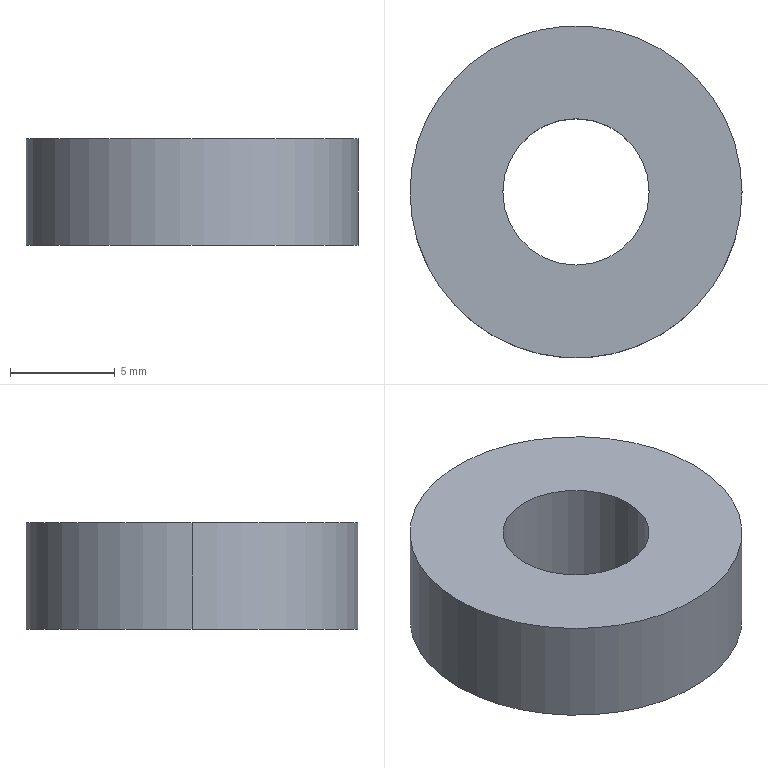Part | STEP file | 1_id982_x_t | 1 solid | 6 faces | box 15.875 x 15.875 x 5.08 mm | volume 809.996 mm3 | cylinder 4 | plane 2 | commonest cylinder face diameters 7 x2 15.875 x2
STEP:
#1=CARTESIAN_POINT('',(0.,0.,0.));
#2=DIRECTION('',(0.,0.,1.));
#3=DIRECTION('',(1.,0.,0.));
#4=AXIS2_PLACEMENT_3D('',#1,#2,#3);
#5=CARTESIAN_POINT('',(263.562,105.,-6.82));
#6=VERTEX_POINT('',#5);
#7=CARTESIAN_POINT('',(263.562,105.,-11.9));
#8=VERTEX_POINT('',#7);
#9=CARTESIAN_POINT('',(263.562,105.,-6.82));
#10=DIRECTION('',(0.,0.,-1.));
#11=VECTOR('',#10,1.);
#12=LINE('',#9,#11);
#13=CARTESIAN_POINT('',(271.5,105.,-6.82));
#14=DIRECTION('',(0.,0.,-1.));
#15=DIRECTION('',(1.,0.,0.));
#16=AXIS2_PLACEMENT_3D('',#13,#14,#15);
#17=CYLINDRICAL_SURFACE('',#16,7.938);
#18=CARTESIAN_POINT('',(3.142,0.));
#19=DIRECTION('',(0.,1.));
#20=VECTOR('',#19,1.);
#21=LINE('',#18,#20);
#22=(GEOMETRIC_REPRESENTATION_CONTEXT(2)PARAMETRIC_REPRESENTATION_CONTEXT()REPRESENTATION_CONTEXT('',''));
#23=DEFINITIONAL_REPRESENTATION('',(#21),#22);
#24=PCURVE('',#17,#23);
#25=CARTESIAN_POINT('',(271.5,105.,-6.82));
#26=DIRECTION('',(0.,0.,-1.));
#27=DIRECTION('',(1.,0.,0.));
#28=AXIS2_PLACEMENT_3D('',#25,#26,#27);
#29=CYLINDRICAL_SURFACE('',#28,7.938);
#30=CARTESIAN_POINT('',(3.142,0.));
#31=DIRECTION('',(0.,1.));
#32=VECTOR('',#31,1.);
#33=LINE('',#30,#32);
#34=(GEOMETRIC_REPRESENTATION_CONTEXT(2)PARAMETRIC_REPRESENTATION_CONTEXT()REPRESENTATION_CONTEXT('',''));
#35=DEFINITIONAL_REPRESENTATION('',(#33),#34);
#36=PCURVE('',#29,#35);
#37=SURFACE_CURVE('',#12,(#24,#36),.PCURVE_S1.);
#38=EDGE_CURVE('',#6,#8,#37,.T.);
#39=ORIENTED_EDGE('',*,*,#38,.F.);
#40=CARTESIAN_POINT('',(279.438,105.,-6.82));
#41=VERTEX_POINT('',#40);
#42=CARTESIAN_POINT('',(271.5,105.,-6.82));
#43=DIRECTION('',(0.,0.,1.));
#44=DIRECTION('',(1.,0.,0.));
#45=AXIS2_PLACEMENT_3D('',#42,#43,#44);
#46=CIRCLE('',#45,7.938);
#47=CARTESIAN_POINT('',(6.283,0.));
#48=DIRECTION('',(-1.,0.));
#49=VECTOR('',#48,1.);
#50=LINE('',#47,#49);
#51=(GEOMETRIC_REPRESENTATION_CONTEXT(2)PARAMETRIC_REPRESENTATION_CONTEXT()REPRESENTATION_CONTEXT('',''));
#52=DEFINITIONAL_REPRESENTATION('',(#50),#51);
#53=PCURVE('',#17,#52);
#54=CARTESIAN_POINT('',(271.5,105.,-6.82));
#55=DIRECTION('',(0.,0.,-1.));
#56=DIRECTION('',(0.,1.,0.));
#57=AXIS2_PLACEMENT_3D('',#54,#55,#56);
#58=PLANE('',#57);
#59=CARTESIAN_POINT('',(0.,7.938));
#60=CARTESIAN_POINT('',(13.748,7.938));
#61=CARTESIAN_POINT('',(6.874,-3.969));
#62=CARTESIAN_POINT('',(0.,-15.875));
#63=CARTESIAN_POINT('',(-6.874,-3.969));
#64=CARTESIAN_POINT('',(-13.748,7.938));
#65=CARTESIAN_POINT('',(0.,7.938));
#66=(BOUNDED_CURVE()B_SPLINE_CURVE(2,(#59,#60,#61,#62,#63,#64,#65),.UNSPECIFIED.,.T.,.F.)B_SPLINE_CURVE_WITH_KNOTS((1,2,2,2,2,1),(-2.094,0.,2.094,4.189,6.283,8.378),.UNSPECIFIED.)CURVE()GEOMETRIC_REPRESENTATION_ITEM()RATIONAL_B_SPLINE_CURVE((1.,0.5,1.,0.5,1.,0.5,1.))REPRESENTATION_ITEM(''));
#67=(GEOMETRIC_REPRESENTATION_CONTEXT(2)PARAMETRIC_REPRESENTATION_CONTEXT()REPRESENTATION_CONTEXT('',''));
#68=DEFINITIONAL_REPRESENTATION('',(#66),#67);
#69=PCURVE('',#58,#68);
#70=SURFACE_CURVE('',#46,(#53,#69),.PCURVE_S1.);
#71=EDGE_CURVE('',#41,#6,#70,.T.);
#72=ORIENTED_EDGE('',*,*,#71,.F.);
#73=CARTESIAN_POINT('',(279.438,105.,-11.9));
#74=VERTEX_POINT('',#73);
#75=CARTESIAN_POINT('',(279.438,105.,-6.82));
#76=DIRECTION('',(0.,0.,1.));
#77=VECTOR('',#76,1.);
#78=LINE('',#75,#77);
#79=CARTESIAN_POINT('',(6.283,0.));
#80=DIRECTION('',(0.,-1.));
#81=VECTOR('',#80,1.);
#82=LINE('',#79,#81);
#83=(GEOMETRIC_REPRESENTATION_CONTEXT(2)PARAMETRIC_REPRESENTATION_CONTEXT()REPRESENTATION_CONTEXT('',''));
#84=DEFINITIONAL_REPRESENTATION('',(#82),#83);
#85=PCURVE('',#17,#84);
#86=CARTESIAN_POINT('',(0.,0.));
#87=DIRECTION('',(0.,-1.));
#88=VECTOR('',#87,1.);
#89=LINE('',#86,#88);
#90=(GEOMETRIC_REPRESENTATION_CONTEXT(2)PARAMETRIC_REPRESENTATION_CONTEXT()REPRESENTATION_CONTEXT('',''));
#91=DEFINITIONAL_REPRESENTATION('',(#89),#90);
#92=PCURVE('',#29,#91);
#93=SURFACE_CURVE('',#78,(#85,#92),.PCURVE_S1.);
#94=EDGE_CURVE('',#74,#41,#93,.T.);
#95=ORIENTED_EDGE('',*,*,#94,.F.);
#96=CARTESIAN_POINT('',(271.5,105.,-11.9));
#97=DIRECTION('',(0.,0.,-1.));
#98=DIRECTION('',(-1.,0.,0.));
#99=AXIS2_PLACEMENT_3D('',#96,#97,#98);
#100=CIRCLE('',#99,7.938);
#101=CARTESIAN_POINT('',(3.142,5.08));
#102=DIRECTION('',(1.,0.));
#103=VECTOR('',#102,1.);
#104=LINE('',#101,#103);
#105=(GEOMETRIC_REPRESENTATION_CONTEXT(2)PARAMETRIC_REPRESENTATION_CONTEXT()REPRESENTATION_CONTEXT('',''));
#106=DEFINITIONAL_REPRESENTATION('',(#104),#105);
#107=PCURVE('',#17,#106);
#108=CARTESIAN_POINT('',(271.5,105.,-11.9));
#109=DIRECTION('',(0.,0.,-1.));
#110=DIRECTION('',(0.,1.,0.));
#111=AXIS2_PLACEMENT_3D('',#108,#109,#110);
#112=PLANE('',#111);
#113=CARTESIAN_POINT('',(0.,0.));
#114=DIRECTION('',(0.,-1.));
#115=AXIS2_PLACEMENT_2D('',#113,#114);
#116=CIRCLE('',#115,7.938);
#117=(GEOMETRIC_REPRESENTATION_CONTEXT(2)PARAMETRIC_REPRESENTATION_CONTEXT()REPRESENTATION_CONTEXT('',''));
#118=DEFINITIONAL_REPRESENTATION('',(#116),#117);
#119=PCURVE('',#112,#118);
#120=SURFACE_CURVE('',#100,(#107,#119),.PCURVE_S1.);
#121=EDGE_CURVE('',#8,#74,#120,.T.);
#122=ORIENTED_EDGE('',*,*,#121,.F.);
#123=EDGE_LOOP('',(#39,#72,#95,#122));
#124=FACE_BOUND('',#123,.T.);
#125=ADVANCED_FACE('',(#124),#17,.T.);
#126=ORIENTED_EDGE('',*,*,#121,.T.);
#127=CARTESIAN_POINT('',(271.5,105.,-11.9));
#128=DIRECTION('',(0.,0.,-1.));
#129=DIRECTION('',(1.,0.,0.));
#130=AXIS2_PLACEMENT_3D('',#127,#128,#129);
#131=CIRCLE('',#130,7.938);
#132=CARTESIAN_POINT('',(0.,0.));
#133=DIRECTION('',(0.,1.));
#134=AXIS2_PLACEMENT_2D('',#132,#133);
#135=CIRCLE('',#134,7.938);
#136=(GEOMETRIC_REPRESENTATION_CONTEXT(2)PARAMETRIC_REPRESENTATION_CONTEXT()REPRESENTATION_CONTEXT('',''));
#137=DEFINITIONAL_REPRESENTATION('',(#135),#136);
#138=PCURVE('',#112,#137);
#139=CARTESIAN_POINT('',(0.,5.08));
#140=DIRECTION('',(1.,0.));
#141=VECTOR('',#140,1.);
#142=LINE('',#139,#141);
#143=(GEOMETRIC_REPRESENTATION_CONTEXT(2)PARAMETRIC_REPRESENTATION_CONTEXT()REPRESENTATION_CONTEXT('',''));
#144=DEFINITIONAL_REPRESENTATION('',(#142),#143);
#145=PCURVE('',#29,#144);
#146=SURFACE_CURVE('',#131,(#138,#145),.PCURVE_S1.);
#147=EDGE_CURVE('',#74,#8,#146,.T.);
#148=ORIENTED_EDGE('',*,*,#147,.T.);
#149=EDGE_LOOP('',(#126,#148));
#150=FACE_BOUND('',#149,.T.);
#151=CARTESIAN_POINT('',(275.,105.,-11.9));
#152=VERTEX_POINT('',#151);
#153=CARTESIAN_POINT('',(268.,105.,-11.9));
#154=VERTEX_POINT('',#153);
#155=CARTESIAN_POINT('',(271.5,105.,-11.9));
#156=DIRECTION('',(0.,0.,1.));
#157=DIRECTION('',(1.,0.,0.));
#158=AXIS2_PLACEMENT_3D('',#155,#156,#157);
#159=CIRCLE('',#158,3.5);
#160=CARTESIAN_POINT('',(0.,3.5));
#161=CARTESIAN_POINT('',(6.062,3.5));
#162=CARTESIAN_POINT('',(3.031,-1.75));
#163=CARTESIAN_POINT('',(0.,-7.));
#164=CARTESIAN_POINT('',(-3.031,-1.75));
#165=CARTESIAN_POINT('',(-6.062,3.5));
#166=CARTESIAN_POINT('',(0.,3.5));
#167=(BOUNDED_CURVE()B_SPLINE_CURVE(2,(#160,#161,#162,#163,#164,#165,#166),.UNSPECIFIED.,.T.,.F.)B_SPLINE_CURVE_WITH_KNOTS((1,2,2,2,2,1),(-2.094,0.,2.094,4.189,6.283,8.378),.UNSPECIFIED.)CURVE()GEOMETRIC_REPRESENTATION_ITEM()RATIONAL_B_SPLINE_CURVE((1.,0.5,1.,0.5,1.,0.5,1.))REPRESENTATION_ITEM(''));
#168=(GEOMETRIC_REPRESENTATION_CONTEXT(2)PARAMETRIC_REPRESENTATION_CONTEXT()REPRESENTATION_CONTEXT('',''));
#169=DEFINITIONAL_REPRESENTATION('',(#167),#168);
#170=PCURVE('',#112,#169);
#171=CARTESIAN_POINT('',(271.5,105.,-11.9));
#172=DIRECTION('',(0.,0.,1.));
#173=DIRECTION('',(-1.,0.,0.));
#174=AXIS2_PLACEMENT_3D('',#171,#172,#173);
#175=CYLINDRICAL_SURFACE('',#174,3.5);
#176=CARTESIAN_POINT('',(3.142,0.));
#177=DIRECTION('',(1.,0.));
#178=VECTOR('',#177,1.);
#179=LINE('',#176,#178);
#180=(GEOMETRIC_REPRESENTATION_CONTEXT(2)PARAMETRIC_REPRESENTATION_CONTEXT()REPRESENTATION_CONTEXT('',''));
#181=DEFINITIONAL_REPRESENTATION('',(#179),#180);
#182=PCURVE('',#175,#181);
#183=SURFACE_CURVE('',#159,(#170,#182),.PCURVE_S1.);
#184=EDGE_CURVE('',#152,#154,#183,.T.);
#185=ORIENTED_EDGE('',*,*,#184,.T.);
#186=CARTESIAN_POINT('',(271.5,105.,-11.9));
#187=DIRECTION('',(0.,0.,1.));
#188=DIRECTION('',(-1.,0.,0.));
#189=AXIS2_PLACEMENT_3D('',#186,#187,#188);
#190=CIRCLE('',#189,3.5);
#191=CARTESIAN_POINT('',(0.,-3.5));
#192=CARTESIAN_POINT('',(-6.062,-3.5));
#193=CARTESIAN_POINT('',(-3.031,1.75));
#194=CARTESIAN_POINT('',(0.,7.));
#195=CARTESIAN_POINT('',(3.031,1.75));
#196=CARTESIAN_POINT('',(6.062,-3.5));
#197=CARTESIAN_POINT('',(0.,-3.5));
#198=(BOUNDED_CURVE()B_SPLINE_CURVE(2,(#191,#192,#193,#194,#195,#196,#197),.UNSPECIFIED.,.T.,.F.)B_SPLINE_CURVE_WITH_KNOTS((1,2,2,2,2,1),(-2.094,0.,2.094,4.189,6.283,8.378),.UNSPECIFIED.)CURVE()GEOMETRIC_REPRESENTATION_ITEM()RATIONAL_B_SPLINE_CURVE((1.,0.5,1.,0.5,1.,0.5,1.))REPRESENTATION_ITEM(''));
#199=(GEOMETRIC_REPRESENTATION_CONTEXT(2)PARAMETRIC_REPRESENTATION_CONTEXT()REPRESENTATION_CONTEXT('',''));
#200=DEFINITIONAL_REPRESENTATION('',(#198),#199);
#201=PCURVE('',#112,#200);
#202=CARTESIAN_POINT('',(271.5,105.,-11.9));
#203=DIRECTION('',(0.,0.,1.));
#204=DIRECTION('',(-1.,0.,0.));
#205=AXIS2_PLACEMENT_3D('',#202,#203,#204);
#206=CYLINDRICAL_SURFACE('',#205,3.5);
#207=CARTESIAN_POINT('',(0.,0.));
#208=DIRECTION('',(1.,0.));
#209=VECTOR('',#208,1.);
#210=LINE('',#207,#209);
#211=(GEOMETRIC_REPRESENTATION_CONTEXT(2)PARAMETRIC_REPRESENTATION_CONTEXT()REPRESENTATION_CONTEXT('',''));
#212=DEFINITIONAL_REPRESENTATION('',(#210),#211);
#213=PCURVE('',#206,#212);
#214=SURFACE_CURVE('',#190,(#201,#213),.PCURVE_S1.);
#215=EDGE_CURVE('',#154,#152,#214,.T.);
#216=ORIENTED_EDGE('',*,*,#215,.T.);
#217=EDGE_LOOP('',(#185,#216));
#218=FACE_BOUND('',#217,.T.);
#219=ADVANCED_FACE('',(#150,#218),#112,.T.);
#220=ORIENTED_EDGE('',*,*,#94,.T.);
#221=CARTESIAN_POINT('',(271.5,105.,-6.82));
#222=DIRECTION('',(0.,0.,1.));
#223=DIRECTION('',(-1.,0.,0.));
#224=AXIS2_PLACEMENT_3D('',#221,#222,#223);
#225=CIRCLE('',#224,7.938);
#226=CARTESIAN_POINT('',(3.142,0.));
#227=DIRECTION('',(-1.,0.));
#228=VECTOR('',#227,1.);
#229=LINE('',#226,#228);
#230=(GEOMETRIC_REPRESENTATION_CONTEXT(2)PARAMETRIC_REPRESENTATION_CONTEXT()REPRESENTATION_CONTEXT('',''));
#231=DEFINITIONAL_REPRESENTATION('',(#229),#230);
#232=PCURVE('',#29,#231);
#233=CARTESIAN_POINT('',(0.,-7.938));
#234=CARTESIAN_POINT('',(-13.748,-7.938));
#235=CARTESIAN_POINT('',(-6.874,3.969));
#236=CARTESIAN_POINT('',(0.,15.875));
#237=CARTESIAN_POINT('',(6.874,3.969));
#238=CARTESIAN_POINT('',(13.748,-7.938));
#239=CARTESIAN_POINT('',(0.,-7.938));
#240=(BOUNDED_CURVE()B_SPLINE_CURVE(2,(#233,#234,#235,#236,#237,#238,#239),.UNSPECIFIED.,.T.,.F.)B_SPLINE_CURVE_WITH_KNOTS((1,2,2,2,2,1),(-2.094,0.,2.094,4.189,6.283,8.378),.UNSPECIFIED.)CURVE()GEOMETRIC_REPRESENTATION_ITEM()RATIONAL_B_SPLINE_CURVE((1.,0.5,1.,0.5,1.,0.5,1.))REPRESENTATION_ITEM(''));
#241=(GEOMETRIC_REPRESENTATION_CONTEXT(2)PARAMETRIC_REPRESENTATION_CONTEXT()REPRESENTATION_CONTEXT('',''));
#242=DEFINITIONAL_REPRESENTATION('',(#240),#241);
#243=PCURVE('',#58,#242);
#244=SURFACE_CURVE('',#225,(#232,#243),.PCURVE_S1.);
#245=EDGE_CURVE('',#6,#41,#244,.T.);
#246=ORIENTED_EDGE('',*,*,#245,.F.);
#247=ORIENTED_EDGE('',*,*,#38,.T.);
#248=ORIENTED_EDGE('',*,*,#147,.F.);
#249=EDGE_LOOP('',(#220,#246,#247,#248));
#250=FACE_BOUND('',#249,.T.);
#251=ADVANCED_FACE('',(#250),#29,.T.);
#252=ORIENTED_EDGE('',*,*,#245,.T.);
#253=ORIENTED_EDGE('',*,*,#71,.T.);
#254=EDGE_LOOP('',(#252,#253));
#255=FACE_BOUND('',#254,.T.);
#256=CARTESIAN_POINT('',(275.,105.,-6.82));
#257=VERTEX_POINT('',#256);
#258=CARTESIAN_POINT('',(268.,105.,-6.82));
#259=VERTEX_POINT('',#258);
#260=CARTESIAN_POINT('',(271.5,105.,-6.82));
#261=DIRECTION('',(0.,0.,-1.));
#262=DIRECTION('',(1.,0.,0.));
#263=AXIS2_PLACEMENT_3D('',#260,#261,#262);
#264=CIRCLE('',#263,3.5);
#265=CARTESIAN_POINT('',(0.,0.));
#266=DIRECTION('',(0.,1.));
#267=AXIS2_PLACEMENT_2D('',#265,#266);
#268=CIRCLE('',#267,3.5);
#269=(GEOMETRIC_REPRESENTATION_CONTEXT(2)PARAMETRIC_REPRESENTATION_CONTEXT()REPRESENTATION_CONTEXT('',''));
#270=DEFINITIONAL_REPRESENTATION('',(#268),#269);
#271=PCURVE('',#58,#270);
#272=CARTESIAN_POINT('',(3.142,5.08));
#273=DIRECTION('',(-1.,0.));
#274=VECTOR('',#273,1.);
#275=LINE('',#272,#274);
#276=(GEOMETRIC_REPRESENTATION_CONTEXT(2)PARAMETRIC_REPRESENTATION_CONTEXT()REPRESENTATION_CONTEXT('',''));
#277=DEFINITIONAL_REPRESENTATION('',(#275),#276);
#278=PCURVE('',#206,#277);
#279=SURFACE_CURVE('',#264,(#271,#278),.PCURVE_S1.);
#280=EDGE_CURVE('',#257,#259,#279,.T.);
#281=ORIENTED_EDGE('',*,*,#280,.T.);
#282=CARTESIAN_POINT('',(271.5,105.,-6.82));
#283=DIRECTION('',(0.,0.,-1.));
#284=DIRECTION('',(-1.,0.,0.));
#285=AXIS2_PLACEMENT_3D('',#282,#283,#284);
#286=CIRCLE('',#285,3.5);
#287=CARTESIAN_POINT('',(0.,0.));
#288=DIRECTION('',(0.,-1.));
#289=AXIS2_PLACEMENT_2D('',#287,#288);
#290=CIRCLE('',#289,3.5);
#291=(GEOMETRIC_REPRESENTATION_CONTEXT(2)PARAMETRIC_REPRESENTATION_CONTEXT()REPRESENTATION_CONTEXT('',''));
#292=DEFINITIONAL_REPRESENTATION('',(#290),#291);
#293=PCURVE('',#58,#292);
#294=CARTESIAN_POINT('',(6.283,5.08));
#295=DIRECTION('',(-1.,0.));
#296=VECTOR('',#295,1.);
#297=LINE('',#294,#296);
#298=(GEOMETRIC_REPRESENTATION_CONTEXT(2)PARAMETRIC_REPRESENTATION_CONTEXT()REPRESENTATION_CONTEXT('',''));
#299=DEFINITIONAL_REPRESENTATION('',(#297),#298);
#300=PCURVE('',#175,#299);
#301=SURFACE_CURVE('',#286,(#293,#300),.PCURVE_S1.);
#302=EDGE_CURVE('',#259,#257,#301,.T.);
#303=ORIENTED_EDGE('',*,*,#302,.T.);
#304=EDGE_LOOP('',(#281,#303));
#305=FACE_BOUND('',#304,.T.);
#306=ADVANCED_FACE('',(#255,#305),#58,.F.);
#307=ORIENTED_EDGE('',*,*,#302,.T.);
#308=CARTESIAN_POINT('',(275.,105.,-11.9));
#309=DIRECTION('',(0.,0.,1.));
#310=VECTOR('',#309,1.);
#311=LINE('',#308,#310);
#312=CARTESIAN_POINT('',(3.142,0.));
#313=DIRECTION('',(0.,1.));
#314=VECTOR('',#313,1.);
#315=LINE('',#312,#314);
#316=(GEOMETRIC_REPRESENTATION_CONTEXT(2)PARAMETRIC_REPRESENTATION_CONTEXT()REPRESENTATION_CONTEXT('',''));
#317=DEFINITIONAL_REPRESENTATION('',(#315),#316);
#318=PCURVE('',#175,#317);
#319=CARTESIAN_POINT('',(3.142,0.));
#320=DIRECTION('',(0.,1.));
#321=VECTOR('',#320,1.);
#322=LINE('',#319,#321);
#323=(GEOMETRIC_REPRESENTATION_CONTEXT(2)PARAMETRIC_REPRESENTATION_CONTEXT()REPRESENTATION_CONTEXT('',''));
#324=DEFINITIONAL_REPRESENTATION('',(#322),#323);
#325=PCURVE('',#206,#324);
#326=SURFACE_CURVE('',#311,(#318,#325),.PCURVE_S1.);
#327=EDGE_CURVE('',#152,#257,#326,.T.);
#328=ORIENTED_EDGE('',*,*,#327,.F.);
#329=ORIENTED_EDGE('',*,*,#184,.T.);
#330=CARTESIAN_POINT('',(268.,105.,-11.9));
#331=DIRECTION('',(0.,0.,-1.));
#332=VECTOR('',#331,1.);
#333=LINE('',#330,#332);
#334=CARTESIAN_POINT('',(6.283,0.));
#335=DIRECTION('',(0.,-1.));
#336=VECTOR('',#335,1.);
#337=LINE('',#334,#336);
#338=(GEOMETRIC_REPRESENTATION_CONTEXT(2)PARAMETRIC_REPRESENTATION_CONTEXT()REPRESENTATION_CONTEXT('',''));
#339=DEFINITIONAL_REPRESENTATION('',(#337),#338);
#340=PCURVE('',#175,#339);
#341=CARTESIAN_POINT('',(0.,0.));
#342=DIRECTION('',(0.,-1.));
#343=VECTOR('',#342,1.);
#344=LINE('',#341,#343);
#345=(GEOMETRIC_REPRESENTATION_CONTEXT(2)PARAMETRIC_REPRESENTATION_CONTEXT()REPRESENTATION_CONTEXT('',''));
#346=DEFINITIONAL_REPRESENTATION('',(#344),#345);
#347=PCURVE('',#206,#346);
#348=SURFACE_CURVE('',#333,(#340,#347),.PCURVE_S1.);
#349=EDGE_CURVE('',#259,#154,#348,.T.);
#350=ORIENTED_EDGE('',*,*,#349,.F.);
#351=EDGE_LOOP('',(#307,#328,#329,#350));
#352=FACE_BOUND('',#351,.F.);
#353=ADVANCED_FACE('',(#352),#175,.F.);
#354=ORIENTED_EDGE('',*,*,#280,.T.);
#355=ORIENTED_EDGE('',*,*,#349,.T.);
#356=ORIENTED_EDGE('',*,*,#215,.T.);
#357=ORIENTED_EDGE('',*,*,#327,.T.);
#358=EDGE_LOOP('',(#354,#355,#356,#357));
#359=FACE_BOUND('',#358,.F.);
#360=ADVANCED_FACE('',(#359),#206,.F.);
#361=CLOSED_SHELL('',(#125,#219,#251,#306,#353,#360));
#362=MANIFOLD_SOLID_BREP('',#361);
#363=(LENGTH_UNIT()NAMED_UNIT(*)SI_UNIT(.MILLI.,.METRE.));
#364=UNCERTAINTY_MEASURE_WITH_UNIT(LENGTH_MEASURE(0.0000001),#363,'','');
#365=(NAMED_UNIT(*)PLANE_ANGLE_UNIT()SI_UNIT($,.RADIAN.));
#366=(NAMED_UNIT(*)SI_UNIT($,.STERADIAN.)SOLID_ANGLE_UNIT());
#367=(GEOMETRIC_REPRESENTATION_CONTEXT(3)GLOBAL_UNCERTAINTY_ASSIGNED_CONTEXT((#364))GLOBAL_UNIT_ASSIGNED_CONTEXT((#363,#365,#366))REPRESENTATION_CONTEXT('',''));
#368=ADVANCED_BREP_SHAPE_REPRESENTATION('',(#4,#362),#367);